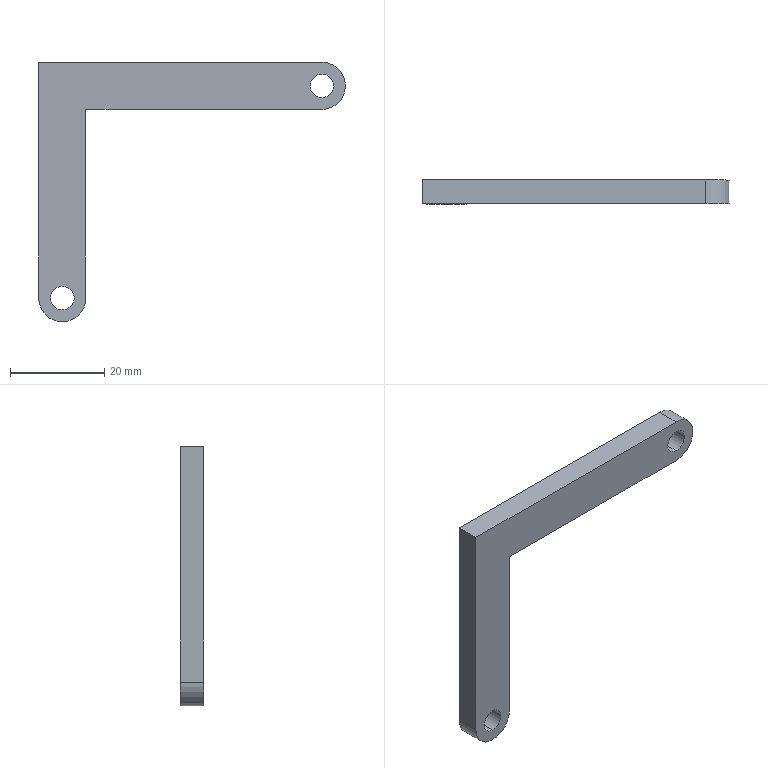Part | SolidWorks | features Extrusion 1 | 1 solid | 13 faces | box 65 x 5 x 55 mm | volume 5196 mm3 | cylinder 7 | plane 6 | commonest cylinder face diameters 5 x4 10 x3
STEP:
#1=CARTESIAN_POINT('',(-30.,5.,-47.5));
#2=VERTEX_POINT('',#1);
#3=CARTESIAN_POINT('',(-30.,5.,-42.5));
#4=VERTEX_POINT('',#3);
#5=CARTESIAN_POINT('',(-30.,5.,-45.));
#6=DIRECTION('',(0.,1.,0.));
#7=DIRECTION('',(0.,0.,1.));
#8=AXIS2_PLACEMENT_3D('',#5,#6,#7);
#9=CIRCLE('',#8,2.5);
#10=EDGE_CURVE('',#2,#4,#9,.T.);
#11=ORIENTED_EDGE('',*,*,#10,.T.);
#12=CARTESIAN_POINT('',(-30.,0.,-42.5));
#13=VERTEX_POINT('',#12);
#14=CARTESIAN_POINT('',(-30.,5.,-42.5));
#15=DIRECTION('',(0.,-1.,0.));
#16=VECTOR('',#15,1000.);
#17=LINE('',#14,#16);
#18=EDGE_CURVE('',#4,#13,#17,.T.);
#19=ORIENTED_EDGE('',*,*,#18,.T.);
#20=CARTESIAN_POINT('',(-30.,0.,-47.5));
#21=VERTEX_POINT('',#20);
#22=CARTESIAN_POINT('',(-30.,0.,-45.));
#23=DIRECTION('',(0.,1.,0.));
#24=DIRECTION('',(0.,0.,1.));
#25=AXIS2_PLACEMENT_3D('',#22,#23,#24);
#26=CIRCLE('',#25,2.5);
#27=EDGE_CURVE('',#21,#13,#26,.T.);
#28=ORIENTED_EDGE('',*,*,#27,.F.);
#29=CARTESIAN_POINT('',(-30.,5.,-47.5));
#30=DIRECTION('',(0.,-1.,0.));
#31=VECTOR('',#30,1000.);
#32=LINE('',#29,#31);
#33=EDGE_CURVE('',#2,#21,#32,.T.);
#34=ORIENTED_EDGE('',*,*,#33,.F.);
#35=EDGE_LOOP('',(#11,#19,#28,#34));
#36=FACE_OUTER_BOUND('',#35,.T.);
#37=CARTESIAN_POINT('',(-30.,5.,-45.));
#38=DIRECTION('',(0.,-1.,0.));
#39=DIRECTION('',(0.,0.,-1.));
#40=AXIS2_PLACEMENT_3D('',#37,#38,#39);
#41=CYLINDRICAL_SURFACE('',#40,2.5);
#42=ADVANCED_FACE('',(#36),#41,.F.);
#43=CARTESIAN_POINT('',(25.,5.,-2.5));
#44=VERTEX_POINT('',#43);
#45=CARTESIAN_POINT('',(25.,5.,2.5));
#46=VERTEX_POINT('',#45);
#47=CARTESIAN_POINT('',(25.,5.,0.));
#48=DIRECTION('',(0.,1.,0.));
#49=DIRECTION('',(0.,0.,1.));
#50=AXIS2_PLACEMENT_3D('',#47,#48,#49);
#51=CIRCLE('',#50,2.5);
#52=EDGE_CURVE('',#44,#46,#51,.T.);
#53=ORIENTED_EDGE('',*,*,#52,.T.);
#54=CARTESIAN_POINT('',(25.,0.,2.5));
#55=VERTEX_POINT('',#54);
#56=CARTESIAN_POINT('',(25.,5.,2.5));
#57=DIRECTION('',(0.,-1.,0.));
#58=VECTOR('',#57,1000.);
#59=LINE('',#56,#58);
#60=EDGE_CURVE('',#46,#55,#59,.T.);
#61=ORIENTED_EDGE('',*,*,#60,.T.);
#62=CARTESIAN_POINT('',(25.,0.,-2.5));
#63=VERTEX_POINT('',#62);
#64=CARTESIAN_POINT('',(25.,0.,0.));
#65=DIRECTION('',(0.,1.,0.));
#66=DIRECTION('',(0.,0.,1.));
#67=AXIS2_PLACEMENT_3D('',#64,#65,#66);
#68=CIRCLE('',#67,2.5);
#69=EDGE_CURVE('',#63,#55,#68,.T.);
#70=ORIENTED_EDGE('',*,*,#69,.F.);
#71=CARTESIAN_POINT('',(25.,5.,-2.5));
#72=DIRECTION('',(0.,-1.,0.));
#73=VECTOR('',#72,1000.);
#74=LINE('',#71,#73);
#75=EDGE_CURVE('',#44,#63,#74,.T.);
#76=ORIENTED_EDGE('',*,*,#75,.F.);
#77=EDGE_LOOP('',(#53,#61,#70,#76));
#78=FACE_OUTER_BOUND('',#77,.T.);
#79=CARTESIAN_POINT('',(25.,5.,0.));
#80=DIRECTION('',(0.,-1.,0.));
#81=DIRECTION('',(0.,0.,-1.));
#82=AXIS2_PLACEMENT_3D('',#79,#80,#81);
#83=CYLINDRICAL_SURFACE('',#82,2.5);
#84=ADVANCED_FACE('',(#78),#83,.F.);
#85=CARTESIAN_POINT('',(-30.,5.,-50.));
#86=VERTEX_POINT('',#85);
#87=CARTESIAN_POINT('',(-35.,5.,-45.));
#88=VERTEX_POINT('',#87);
#89=CARTESIAN_POINT('',(-30.,5.,-45.));
#90=DIRECTION('',(0.,1.,0.));
#91=DIRECTION('',(0.,0.,1.));
#92=AXIS2_PLACEMENT_3D('',#89,#90,#91);
#93=CIRCLE('',#92,5.);
#94=EDGE_CURVE('',#86,#88,#93,.T.);
#95=ORIENTED_EDGE('',*,*,#94,.F.);
#96=CARTESIAN_POINT('',(-30.,0.,-50.));
#97=VERTEX_POINT('',#96);
#98=CARTESIAN_POINT('',(-30.,5.,-50.));
#99=DIRECTION('',(0.,-1.,0.));
#100=VECTOR('',#99,1000.);
#101=LINE('',#98,#100);
#102=EDGE_CURVE('',#86,#97,#101,.T.);
#103=ORIENTED_EDGE('',*,*,#102,.T.);
#104=CARTESIAN_POINT('',(-35.,0.,-45.));
#105=VERTEX_POINT('',#104);
#106=CARTESIAN_POINT('',(-30.,0.,-45.));
#107=DIRECTION('',(0.,1.,0.));
#108=DIRECTION('',(0.,0.,1.));
#109=AXIS2_PLACEMENT_3D('',#106,#107,#108);
#110=CIRCLE('',#109,5.);
#111=EDGE_CURVE('',#97,#105,#110,.T.);
#112=ORIENTED_EDGE('',*,*,#111,.T.);
#113=CARTESIAN_POINT('',(-35.,5.,-45.));
#114=DIRECTION('',(0.,-1.,0.));
#115=VECTOR('',#114,1000.);
#116=LINE('',#113,#115);
#117=EDGE_CURVE('',#88,#105,#116,.T.);
#118=ORIENTED_EDGE('',*,*,#117,.F.);
#119=EDGE_LOOP('',(#95,#103,#112,#118));
#120=FACE_OUTER_BOUND('',#119,.T.);
#121=CARTESIAN_POINT('',(-30.,5.,-45.));
#122=DIRECTION('',(0.,-1.,0.));
#123=DIRECTION('',(0.,0.,-1.));
#124=AXIS2_PLACEMENT_3D('',#121,#122,#123);
#125=CYLINDRICAL_SURFACE('',#124,5.);
#126=ADVANCED_FACE('',(#120),#125,.T.);
#127=ORIENTED_EDGE('',*,*,#52,.F.);
#128=CARTESIAN_POINT('',(25.,5.,0.));
#129=DIRECTION('',(0.,1.,0.));
#130=DIRECTION('',(0.,0.,1.));
#131=AXIS2_PLACEMENT_3D('',#128,#129,#130);
#132=CIRCLE('',#131,2.5);
#133=EDGE_CURVE('',#46,#44,#132,.T.);
#134=ORIENTED_EDGE('',*,*,#133,.F.);
#135=EDGE_LOOP('',(#127,#134));
#136=FACE_BOUND('',#135,.T.);
#137=CARTESIAN_POINT('',(25.,5.,5.));
#138=VERTEX_POINT('',#137);
#139=CARTESIAN_POINT('',(25.,5.,-5.));
#140=VERTEX_POINT('',#139);
#141=CARTESIAN_POINT('',(25.,5.,0.));
#142=DIRECTION('',(0.,1.,0.));
#143=DIRECTION('',(0.,0.,1.));
#144=AXIS2_PLACEMENT_3D('',#141,#142,#143);
#145=CIRCLE('',#144,5.);
#146=EDGE_CURVE('',#138,#140,#145,.T.);
#147=ORIENTED_EDGE('',*,*,#146,.T.);
#148=CARTESIAN_POINT('',(-25.,5.,-5.));
#149=VERTEX_POINT('',#148);
#150=CARTESIAN_POINT('',(-25.,5.,-5.));
#151=DIRECTION('',(-1.,0.,0.));
#152=VECTOR('',#151,1000.);
#153=LINE('',#150,#152);
#154=EDGE_CURVE('',#140,#149,#153,.T.);
#155=ORIENTED_EDGE('',*,*,#154,.T.);
#156=CARTESIAN_POINT('',(-25.,5.,-45.));
#157=VERTEX_POINT('',#156);
#158=CARTESIAN_POINT('',(-25.,5.,-5.));
#159=DIRECTION('',(0.,0.,-1.));
#160=VECTOR('',#159,1000.);
#161=LINE('',#158,#160);
#162=EDGE_CURVE('',#149,#157,#161,.T.);
#163=ORIENTED_EDGE('',*,*,#162,.T.);
#164=CARTESIAN_POINT('',(-30.,5.,-45.));
#165=DIRECTION('',(0.,1.,0.));
#166=DIRECTION('',(0.,0.,1.));
#167=AXIS2_PLACEMENT_3D('',#164,#165,#166);
#168=CIRCLE('',#167,5.);
#169=EDGE_CURVE('',#157,#86,#168,.T.);
#170=ORIENTED_EDGE('',*,*,#169,.T.);
#171=ORIENTED_EDGE('',*,*,#94,.T.);
#172=CARTESIAN_POINT('',(-35.,5.,5.));
#173=VERTEX_POINT('',#172);
#174=CARTESIAN_POINT('',(-35.,5.,5.));
#175=DIRECTION('',(0.,0.,1.));
#176=VECTOR('',#175,1000.);
#177=LINE('',#174,#176);
#178=EDGE_CURVE('',#88,#173,#177,.T.);
#179=ORIENTED_EDGE('',*,*,#178,.T.);
#180=CARTESIAN_POINT('',(-25.,5.,5.));
#181=DIRECTION('',(1.,0.,0.));
#182=VECTOR('',#181,1000.);
#183=LINE('',#180,#182);
#184=EDGE_CURVE('',#173,#138,#183,.T.);
#185=ORIENTED_EDGE('',*,*,#184,.T.);
#186=EDGE_LOOP('',(#147,#155,#163,#170,#171,#179,#185));
#187=FACE_OUTER_BOUND('',#186,.T.);
#188=ORIENTED_EDGE('',*,*,#10,.F.);
#189=CARTESIAN_POINT('',(-30.,5.,-45.));
#190=DIRECTION('',(0.,1.,0.));
#191=DIRECTION('',(0.,0.,1.));
#192=AXIS2_PLACEMENT_3D('',#189,#190,#191);
#193=CIRCLE('',#192,2.5);
#194=EDGE_CURVE('',#4,#2,#193,.T.);
#195=ORIENTED_EDGE('',*,*,#194,.F.);
#196=EDGE_LOOP('',(#188,#195));
#197=FACE_BOUND('',#196,.T.);
#198=CARTESIAN_POINT('',(25.,5.,0.));
#199=DIRECTION('',(0.,1.,0.));
#200=DIRECTION('',(0.,0.,1.));
#201=AXIS2_PLACEMENT_3D('',#198,#199,#200);
#202=PLANE('',#201);
#203=ADVANCED_FACE('',(#136,#187,#197),#202,.T.);
#204=CARTESIAN_POINT('',(25.,0.,5.));
#205=VERTEX_POINT('',#204);
#206=CARTESIAN_POINT('',(25.,0.,-5.));
#207=VERTEX_POINT('',#206);
#208=CARTESIAN_POINT('',(25.,0.,0.));
#209=DIRECTION('',(0.,1.,0.));
#210=DIRECTION('',(0.,0.,1.));
#211=AXIS2_PLACEMENT_3D('',#208,#209,#210);
#212=CIRCLE('',#211,5.);
#213=EDGE_CURVE('',#205,#207,#212,.T.);
#214=ORIENTED_EDGE('',*,*,#213,.F.);
#215=CARTESIAN_POINT('',(-35.,0.,5.));
#216=VERTEX_POINT('',#215);
#217=CARTESIAN_POINT('',(-25.,0.,5.));
#218=DIRECTION('',(1.,0.,0.));
#219=VECTOR('',#218,1000.);
#220=LINE('',#217,#219);
#221=EDGE_CURVE('',#216,#205,#220,.T.);
#222=ORIENTED_EDGE('',*,*,#221,.F.);
#223=CARTESIAN_POINT('',(-35.,0.,5.));
#224=DIRECTION('',(0.,0.,1.));
#225=VECTOR('',#224,1000.);
#226=LINE('',#223,#225);
#227=EDGE_CURVE('',#105,#216,#226,.T.);
#228=ORIENTED_EDGE('',*,*,#227,.F.);
#229=ORIENTED_EDGE('',*,*,#111,.F.);
#230=CARTESIAN_POINT('',(-25.,0.,-45.));
#231=VERTEX_POINT('',#230);
#232=CARTESIAN_POINT('',(-30.,0.,-45.));
#233=DIRECTION('',(0.,1.,0.));
#234=DIRECTION('',(0.,0.,1.));
#235=AXIS2_PLACEMENT_3D('',#232,#233,#234);
#236=CIRCLE('',#235,5.);
#237=EDGE_CURVE('',#231,#97,#236,.T.);
#238=ORIENTED_EDGE('',*,*,#237,.F.);
#239=CARTESIAN_POINT('',(-25.,0.,-5.));
#240=VERTEX_POINT('',#239);
#241=CARTESIAN_POINT('',(-25.,0.,-5.));
#242=DIRECTION('',(0.,0.,-1.));
#243=VECTOR('',#242,1000.);
#244=LINE('',#241,#243);
#245=EDGE_CURVE('',#240,#231,#244,.T.);
#246=ORIENTED_EDGE('',*,*,#245,.F.);
#247=CARTESIAN_POINT('',(-25.,0.,-5.));
#248=DIRECTION('',(-1.,0.,0.));
#249=VECTOR('',#248,1000.);
#250=LINE('',#247,#249);
#251=EDGE_CURVE('',#207,#240,#250,.T.);
#252=ORIENTED_EDGE('',*,*,#251,.F.);
#253=EDGE_LOOP('',(#214,#222,#228,#229,#238,#246,#252));
#254=FACE_OUTER_BOUND('',#253,.T.);
#255=ORIENTED_EDGE('',*,*,#69,.T.);
#256=CARTESIAN_POINT('',(25.,0.,0.));
#257=DIRECTION('',(0.,1.,0.));
#258=DIRECTION('',(0.,0.,1.));
#259=AXIS2_PLACEMENT_3D('',#256,#257,#258);
#260=CIRCLE('',#259,2.5);
#261=EDGE_CURVE('',#55,#63,#260,.T.);
#262=ORIENTED_EDGE('',*,*,#261,.T.);
#263=EDGE_LOOP('',(#255,#262));
#264=FACE_BOUND('',#263,.T.);
#265=ORIENTED_EDGE('',*,*,#27,.T.);
#266=CARTESIAN_POINT('',(-30.,0.,-45.));
#267=DIRECTION('',(0.,1.,0.));
#268=DIRECTION('',(0.,0.,1.));
#269=AXIS2_PLACEMENT_3D('',#266,#267,#268);
#270=CIRCLE('',#269,2.5);
#271=EDGE_CURVE('',#13,#21,#270,.T.);
#272=ORIENTED_EDGE('',*,*,#271,.T.);
#273=EDGE_LOOP('',(#265,#272));
#274=FACE_BOUND('',#273,.T.);
#275=CARTESIAN_POINT('',(25.,0.,0.));
#276=DIRECTION('',(0.,1.,0.));
#277=DIRECTION('',(0.,0.,1.));
#278=AXIS2_PLACEMENT_3D('',#275,#276,#277);
#279=PLANE('',#278);
#280=ADVANCED_FACE('',(#254,#264,#274),#279,.F.);
#281=ORIENTED_EDGE('',*,*,#213,.T.);
#282=CARTESIAN_POINT('',(25.,5.,-5.));
#283=DIRECTION('',(0.,-1.,0.));
#284=VECTOR('',#283,1000.);
#285=LINE('',#282,#284);
#286=EDGE_CURVE('',#140,#207,#285,.T.);
#287=ORIENTED_EDGE('',*,*,#286,.F.);
#288=ORIENTED_EDGE('',*,*,#146,.F.);
#289=CARTESIAN_POINT('',(25.,5.,5.));
#290=DIRECTION('',(0.,-1.,0.));
#291=VECTOR('',#290,1000.);
#292=LINE('',#289,#291);
#293=EDGE_CURVE('',#138,#205,#292,.T.);
#294=ORIENTED_EDGE('',*,*,#293,.T.);
#295=EDGE_LOOP('',(#281,#287,#288,#294));
#296=FACE_OUTER_BOUND('',#295,.T.);
#297=CARTESIAN_POINT('',(25.,5.,0.));
#298=DIRECTION('',(0.,-1.,0.));
#299=DIRECTION('',(0.,0.,-1.));
#300=AXIS2_PLACEMENT_3D('',#297,#298,#299);
#301=CYLINDRICAL_SURFACE('',#300,5.);
#302=ADVANCED_FACE('',(#296),#301,.T.);
#303=ORIENTED_EDGE('',*,*,#251,.T.);
#304=CARTESIAN_POINT('',(-25.,5.,-5.));
#305=DIRECTION('',(0.,-1.,0.));
#306=VECTOR('',#305,1000.);
#307=LINE('',#304,#306);
#308=EDGE_CURVE('',#149,#240,#307,.T.);
#309=ORIENTED_EDGE('',*,*,#308,.F.);
#310=ORIENTED_EDGE('',*,*,#154,.F.);
#311=ORIENTED_EDGE('',*,*,#286,.T.);
#312=EDGE_LOOP('',(#303,#309,#310,#311));
#313=FACE_OUTER_BOUND('',#312,.T.);
#314=CARTESIAN_POINT('',(-25.,5.,-5.));
#315=DIRECTION('',(0.,0.,1.));
#316=DIRECTION('',(1.,0.,0.));
#317=AXIS2_PLACEMENT_3D('',#314,#315,#316);
#318=PLANE('',#317);
#319=ADVANCED_FACE('',(#313),#318,.F.);
#320=ORIENTED_EDGE('',*,*,#245,.T.);
#321=CARTESIAN_POINT('',(-25.,5.,-45.));
#322=DIRECTION('',(0.,-1.,0.));
#323=VECTOR('',#322,1000.);
#324=LINE('',#321,#323);
#325=EDGE_CURVE('',#157,#231,#324,.T.);
#326=ORIENTED_EDGE('',*,*,#325,.F.);
#327=ORIENTED_EDGE('',*,*,#162,.F.);
#328=ORIENTED_EDGE('',*,*,#308,.T.);
#329=EDGE_LOOP('',(#320,#326,#327,#328));
#330=FACE_OUTER_BOUND('',#329,.T.);
#331=CARTESIAN_POINT('',(-25.,5.,-5.));
#332=DIRECTION('',(-1.,0.,0.));
#333=DIRECTION('',(0.,0.,1.));
#334=AXIS2_PLACEMENT_3D('',#331,#332,#333);
#335=PLANE('',#334);
#336=ADVANCED_FACE('',(#330),#335,.F.);
#337=ORIENTED_EDGE('',*,*,#102,.F.);
#338=ORIENTED_EDGE('',*,*,#169,.F.);
#339=ORIENTED_EDGE('',*,*,#325,.T.);
#340=ORIENTED_EDGE('',*,*,#237,.T.);
#341=EDGE_LOOP('',(#337,#338,#339,#340));
#342=FACE_OUTER_BOUND('',#341,.T.);
#343=CARTESIAN_POINT('',(-30.,5.,-45.));
#344=DIRECTION('',(0.,-1.,0.));
#345=DIRECTION('',(0.,0.,-1.));
#346=AXIS2_PLACEMENT_3D('',#343,#344,#345);
#347=CYLINDRICAL_SURFACE('',#346,5.);
#348=ADVANCED_FACE('',(#342),#347,.T.);
#349=ORIENTED_EDGE('',*,*,#227,.T.);
#350=CARTESIAN_POINT('',(-35.,5.,5.));
#351=DIRECTION('',(0.,-1.,0.));
#352=VECTOR('',#351,1000.);
#353=LINE('',#350,#352);
#354=EDGE_CURVE('',#173,#216,#353,.T.);
#355=ORIENTED_EDGE('',*,*,#354,.F.);
#356=ORIENTED_EDGE('',*,*,#178,.F.);
#357=ORIENTED_EDGE('',*,*,#117,.T.);
#358=EDGE_LOOP('',(#349,#355,#356,#357));
#359=FACE_OUTER_BOUND('',#358,.T.);
#360=CARTESIAN_POINT('',(-35.,5.,5.));
#361=DIRECTION('',(1.,0.,0.));
#362=DIRECTION('',(0.,0.,-1.));
#363=AXIS2_PLACEMENT_3D('',#360,#361,#362);
#364=PLANE('',#363);
#365=ADVANCED_FACE('',(#359),#364,.F.);
#366=ORIENTED_EDGE('',*,*,#221,.T.);
#367=ORIENTED_EDGE('',*,*,#293,.F.);
#368=ORIENTED_EDGE('',*,*,#184,.F.);
#369=ORIENTED_EDGE('',*,*,#354,.T.);
#370=EDGE_LOOP('',(#366,#367,#368,#369));
#371=FACE_OUTER_BOUND('',#370,.T.);
#372=CARTESIAN_POINT('',(-25.,5.,5.));
#373=DIRECTION('',(0.,0.,-1.));
#374=DIRECTION('',(-1.,0.,0.));
#375=AXIS2_PLACEMENT_3D('',#372,#373,#374);
#376=PLANE('',#375);
#377=ADVANCED_FACE('',(#371),#376,.F.);
#378=ORIENTED_EDGE('',*,*,#60,.F.);
#379=ORIENTED_EDGE('',*,*,#133,.T.);
#380=ORIENTED_EDGE('',*,*,#75,.T.);
#381=ORIENTED_EDGE('',*,*,#261,.F.);
#382=EDGE_LOOP('',(#378,#379,#380,#381));
#383=FACE_OUTER_BOUND('',#382,.T.);
#384=CARTESIAN_POINT('',(25.,5.,0.));
#385=DIRECTION('',(0.,-1.,0.));
#386=DIRECTION('',(0.,0.,-1.));
#387=AXIS2_PLACEMENT_3D('',#384,#385,#386);
#388=CYLINDRICAL_SURFACE('',#387,2.5);
#389=ADVANCED_FACE('',(#383),#388,.F.);
#390=ORIENTED_EDGE('',*,*,#18,.F.);
#391=ORIENTED_EDGE('',*,*,#194,.T.);
#392=ORIENTED_EDGE('',*,*,#33,.T.);
#393=ORIENTED_EDGE('',*,*,#271,.F.);
#394=EDGE_LOOP('',(#390,#391,#392,#393));
#395=FACE_OUTER_BOUND('',#394,.T.);
#396=CARTESIAN_POINT('',(-30.,5.,-45.));
#397=DIRECTION('',(0.,-1.,0.));
#398=DIRECTION('',(0.,0.,-1.));
#399=AXIS2_PLACEMENT_3D('',#396,#397,#398);
#400=CYLINDRICAL_SURFACE('',#399,2.5);
#401=ADVANCED_FACE('',(#395),#400,.F.);
#402=CLOSED_SHELL('',(#42,#84,#126,#203,#280,#302,#319,#336,#348,#365,#377,#389,#401));
#403=MANIFOLD_SOLID_BREP('',#402);
#404=CARTESIAN_POINT('',(0.,0.,0.));
#405=DIRECTION('',(0.,0.,1.));
#406=DIRECTION('',(1.,0.,0.));
#407=AXIS2_PLACEMENT_3D('',#404,#405,#406);
#408=(LENGTH_UNIT()NAMED_UNIT(*)SI_UNIT(.MILLI.,.METRE.));
#409=UNCERTAINTY_MEASURE_WITH_UNIT(LENGTH_MEASURE(0.00001),#408,'','');
#410=(NAMED_UNIT(*)PLANE_ANGLE_UNIT()SI_UNIT($,.RADIAN.));
#411=(NAMED_UNIT(*)SI_UNIT($,.STERADIAN.)SOLID_ANGLE_UNIT());
#412=(GEOMETRIC_REPRESENTATION_CONTEXT(3)GLOBAL_UNCERTAINTY_ASSIGNED_CONTEXT((#409))GLOBAL_UNIT_ASSIGNED_CONTEXT((#408,#410,#411))REPRESENTATION_CONTEXT('',''));
#413=ADVANCED_BREP_SHAPE_REPRESENTATION('',(#403,#407),#412);